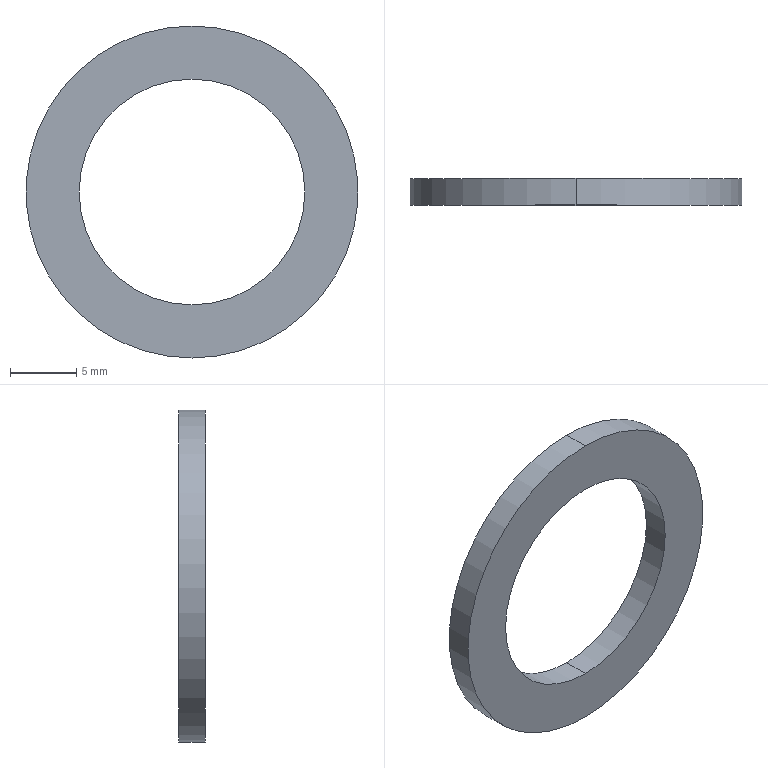Part | SolidWorks | features Extrusion 1 | 1 solid | 6 faces | box 25 x 2 x 25 mm | volume 527.788 mm3 | cylinder 4 | plane 2 | commonest cylinder face diameters 17 x2 25 x2
STEP:
#1=CARTESIAN_POINT('',(0.,2.,-8.5));
#2=VERTEX_POINT('',#1);
#3=CARTESIAN_POINT('',(0.,2.,8.5));
#4=VERTEX_POINT('',#3);
#5=CARTESIAN_POINT('',(0.,2.,0.));
#6=DIRECTION('',(0.,1.,0.));
#7=DIRECTION('',(0.,0.,1.));
#8=AXIS2_PLACEMENT_3D('',#5,#6,#7);
#9=CIRCLE('',#8,8.5);
#10=EDGE_CURVE('',#2,#4,#9,.T.);
#11=ORIENTED_EDGE('',*,*,#10,.T.);
#12=CARTESIAN_POINT('',(0.,0.,8.5));
#13=VERTEX_POINT('',#12);
#14=CARTESIAN_POINT('',(0.,2.,8.5));
#15=DIRECTION('',(0.,-1.,0.));
#16=VECTOR('',#15,1000.);
#17=LINE('',#14,#16);
#18=EDGE_CURVE('',#4,#13,#17,.T.);
#19=ORIENTED_EDGE('',*,*,#18,.T.);
#20=CARTESIAN_POINT('',(0.,0.,-8.5));
#21=VERTEX_POINT('',#20);
#22=CARTESIAN_POINT('',(0.,0.,0.));
#23=DIRECTION('',(0.,1.,0.));
#24=DIRECTION('',(0.,0.,1.));
#25=AXIS2_PLACEMENT_3D('',#22,#23,#24);
#26=CIRCLE('',#25,8.5);
#27=EDGE_CURVE('',#21,#13,#26,.T.);
#28=ORIENTED_EDGE('',*,*,#27,.F.);
#29=CARTESIAN_POINT('',(0.,2.,-8.5));
#30=DIRECTION('',(0.,-1.,0.));
#31=VECTOR('',#30,1000.);
#32=LINE('',#29,#31);
#33=EDGE_CURVE('',#2,#21,#32,.T.);
#34=ORIENTED_EDGE('',*,*,#33,.F.);
#35=EDGE_LOOP('',(#11,#19,#28,#34));
#36=FACE_OUTER_BOUND('',#35,.T.);
#37=CARTESIAN_POINT('',(0.,2.,0.));
#38=DIRECTION('',(0.,-1.,0.));
#39=DIRECTION('',(0.,0.,-1.));
#40=AXIS2_PLACEMENT_3D('',#37,#38,#39);
#41=CYLINDRICAL_SURFACE('',#40,8.5);
#42=ADVANCED_FACE('',(#36),#41,.F.);
#43=CARTESIAN_POINT('',(0.,2.,12.5));
#44=VERTEX_POINT('',#43);
#45=CARTESIAN_POINT('',(0.,2.,-12.5));
#46=VERTEX_POINT('',#45);
#47=CARTESIAN_POINT('',(0.,2.,0.));
#48=DIRECTION('',(0.,1.,0.));
#49=DIRECTION('',(0.,0.,1.));
#50=AXIS2_PLACEMENT_3D('',#47,#48,#49);
#51=CIRCLE('',#50,12.5);
#52=EDGE_CURVE('',#44,#46,#51,.T.);
#53=ORIENTED_EDGE('',*,*,#52,.F.);
#54=CARTESIAN_POINT('',(0.,0.,12.5));
#55=VERTEX_POINT('',#54);
#56=CARTESIAN_POINT('',(0.,2.,12.5));
#57=DIRECTION('',(0.,-1.,0.));
#58=VECTOR('',#57,1000.);
#59=LINE('',#56,#58);
#60=EDGE_CURVE('',#44,#55,#59,.T.);
#61=ORIENTED_EDGE('',*,*,#60,.T.);
#62=CARTESIAN_POINT('',(0.,0.,-12.5));
#63=VERTEX_POINT('',#62);
#64=CARTESIAN_POINT('',(0.,0.,0.));
#65=DIRECTION('',(0.,1.,0.));
#66=DIRECTION('',(0.,0.,1.));
#67=AXIS2_PLACEMENT_3D('',#64,#65,#66);
#68=CIRCLE('',#67,12.5);
#69=EDGE_CURVE('',#55,#63,#68,.T.);
#70=ORIENTED_EDGE('',*,*,#69,.T.);
#71=CARTESIAN_POINT('',(0.,2.,-12.5));
#72=DIRECTION('',(0.,-1.,0.));
#73=VECTOR('',#72,1000.);
#74=LINE('',#71,#73);
#75=EDGE_CURVE('',#46,#63,#74,.T.);
#76=ORIENTED_EDGE('',*,*,#75,.F.);
#77=EDGE_LOOP('',(#53,#61,#70,#76));
#78=FACE_OUTER_BOUND('',#77,.T.);
#79=CARTESIAN_POINT('',(0.,2.,0.));
#80=DIRECTION('',(0.,-1.,0.));
#81=DIRECTION('',(0.,0.,-1.));
#82=AXIS2_PLACEMENT_3D('',#79,#80,#81);
#83=CYLINDRICAL_SURFACE('',#82,12.5);
#84=ADVANCED_FACE('',(#78),#83,.T.);
#85=CARTESIAN_POINT('',(0.,2.,0.));
#86=DIRECTION('',(0.,1.,0.));
#87=DIRECTION('',(0.,0.,1.));
#88=AXIS2_PLACEMENT_3D('',#85,#86,#87);
#89=CIRCLE('',#88,12.5);
#90=EDGE_CURVE('',#46,#44,#89,.T.);
#91=ORIENTED_EDGE('',*,*,#90,.T.);
#92=ORIENTED_EDGE('',*,*,#52,.T.);
#93=EDGE_LOOP('',(#91,#92));
#94=FACE_OUTER_BOUND('',#93,.T.);
#95=ORIENTED_EDGE('',*,*,#10,.F.);
#96=CARTESIAN_POINT('',(0.,2.,0.));
#97=DIRECTION('',(0.,1.,0.));
#98=DIRECTION('',(0.,0.,1.));
#99=AXIS2_PLACEMENT_3D('',#96,#97,#98);
#100=CIRCLE('',#99,8.5);
#101=EDGE_CURVE('',#4,#2,#100,.T.);
#102=ORIENTED_EDGE('',*,*,#101,.F.);
#103=EDGE_LOOP('',(#95,#102));
#104=FACE_BOUND('',#103,.T.);
#105=CARTESIAN_POINT('',(0.,2.,0.));
#106=DIRECTION('',(0.,1.,0.));
#107=DIRECTION('',(0.,0.,1.));
#108=AXIS2_PLACEMENT_3D('',#105,#106,#107);
#109=PLANE('',#108);
#110=ADVANCED_FACE('',(#94,#104),#109,.T.);
#111=CARTESIAN_POINT('',(0.,0.,0.));
#112=DIRECTION('',(0.,1.,0.));
#113=DIRECTION('',(0.,0.,1.));
#114=AXIS2_PLACEMENT_3D('',#111,#112,#113);
#115=CIRCLE('',#114,12.5);
#116=EDGE_CURVE('',#63,#55,#115,.T.);
#117=ORIENTED_EDGE('',*,*,#116,.F.);
#118=ORIENTED_EDGE('',*,*,#69,.F.);
#119=EDGE_LOOP('',(#117,#118));
#120=FACE_OUTER_BOUND('',#119,.T.);
#121=ORIENTED_EDGE('',*,*,#27,.T.);
#122=CARTESIAN_POINT('',(0.,0.,0.));
#123=DIRECTION('',(0.,1.,0.));
#124=DIRECTION('',(0.,0.,1.));
#125=AXIS2_PLACEMENT_3D('',#122,#123,#124);
#126=CIRCLE('',#125,8.5);
#127=EDGE_CURVE('',#13,#21,#126,.T.);
#128=ORIENTED_EDGE('',*,*,#127,.T.);
#129=EDGE_LOOP('',(#121,#128));
#130=FACE_BOUND('',#129,.T.);
#131=CARTESIAN_POINT('',(0.,0.,0.));
#132=DIRECTION('',(0.,1.,0.));
#133=DIRECTION('',(0.,0.,1.));
#134=AXIS2_PLACEMENT_3D('',#131,#132,#133);
#135=PLANE('',#134);
#136=ADVANCED_FACE('',(#120,#130),#135,.F.);
#137=ORIENTED_EDGE('',*,*,#60,.F.);
#138=ORIENTED_EDGE('',*,*,#90,.F.);
#139=ORIENTED_EDGE('',*,*,#75,.T.);
#140=ORIENTED_EDGE('',*,*,#116,.T.);
#141=EDGE_LOOP('',(#137,#138,#139,#140));
#142=FACE_OUTER_BOUND('',#141,.T.);
#143=CARTESIAN_POINT('',(0.,2.,0.));
#144=DIRECTION('',(0.,-1.,0.));
#145=DIRECTION('',(0.,0.,-1.));
#146=AXIS2_PLACEMENT_3D('',#143,#144,#145);
#147=CYLINDRICAL_SURFACE('',#146,12.5);
#148=ADVANCED_FACE('',(#142),#147,.T.);
#149=ORIENTED_EDGE('',*,*,#18,.F.);
#150=ORIENTED_EDGE('',*,*,#101,.T.);
#151=ORIENTED_EDGE('',*,*,#33,.T.);
#152=ORIENTED_EDGE('',*,*,#127,.F.);
#153=EDGE_LOOP('',(#149,#150,#151,#152));
#154=FACE_OUTER_BOUND('',#153,.T.);
#155=CARTESIAN_POINT('',(0.,2.,0.));
#156=DIRECTION('',(0.,-1.,0.));
#157=DIRECTION('',(0.,0.,-1.));
#158=AXIS2_PLACEMENT_3D('',#155,#156,#157);
#159=CYLINDRICAL_SURFACE('',#158,8.5);
#160=ADVANCED_FACE('',(#154),#159,.F.);
#161=CLOSED_SHELL('',(#42,#84,#110,#136,#148,#160));
#162=MANIFOLD_SOLID_BREP('',#161);
#163=CARTESIAN_POINT('',(0.,0.,0.));
#164=DIRECTION('',(0.,0.,1.));
#165=DIRECTION('',(1.,0.,0.));
#166=AXIS2_PLACEMENT_3D('',#163,#164,#165);
#167=(LENGTH_UNIT()NAMED_UNIT(*)SI_UNIT(.MILLI.,.METRE.));
#168=UNCERTAINTY_MEASURE_WITH_UNIT(LENGTH_MEASURE(0.00001),#167,'','');
#169=(NAMED_UNIT(*)PLANE_ANGLE_UNIT()SI_UNIT($,.RADIAN.));
#170=(NAMED_UNIT(*)SI_UNIT($,.STERADIAN.)SOLID_ANGLE_UNIT());
#171=(GEOMETRIC_REPRESENTATION_CONTEXT(3)GLOBAL_UNCERTAINTY_ASSIGNED_CONTEXT((#168))GLOBAL_UNIT_ASSIGNED_CONTEXT((#167,#169,#170))REPRESENTATION_CONTEXT('',''));
#172=ADVANCED_BREP_SHAPE_REPRESENTATION('',(#162,#166),#171);